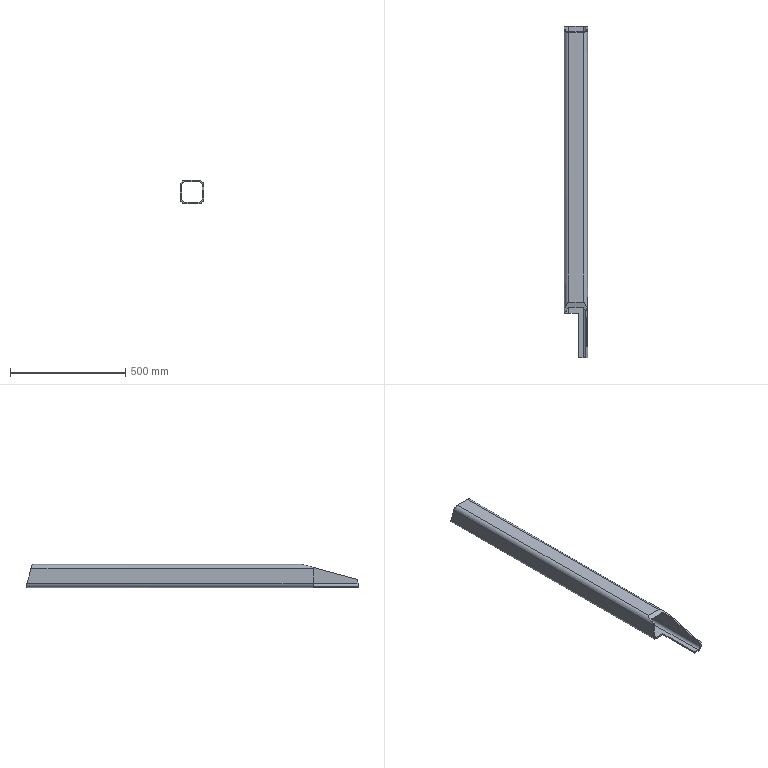Part | SolidWorks | features MirrorStock 1 | 1 solid | 21 faces | box 100 x 1442 x 100 mm | volume 2662768 mm3 | plane 13 | cylinder 8 | commonest cylinder face diameters 26.12 x4 38.12 x4
STEP:
#1=CARTESIAN_POINT('',(-50.,1420.107,30.94));
#2=VERTEX_POINT('',#1);
#3=CARTESIAN_POINT('',(-69.06,1415.,50.));
#4=VERTEX_POINT('',#3);
#5=CARTESIAN_POINT('',(-50.,1420.107,30.94));
#6=CARTESIAN_POINT('',(-50.,1417.115,42.105));
#7=CARTESIAN_POINT('',(-57.895,1415.,50.));
#8=CARTESIAN_POINT('',(-69.06,1415.,50.));
#9=(BOUNDED_CURVE()B_SPLINE_CURVE(3,(#5,#6,#7,#8),.UNSPECIFIED.,.F.,.T.)B_SPLINE_CURVE_WITH_KNOTS((4,4),(4.712,6.283),.UNSPECIFIED.)CURVE()GEOMETRIC_REPRESENTATION_ITEM()RATIONAL_B_SPLINE_CURVE((1.,0.8047,0.8047,1.))REPRESENTATION_ITEM(''));
#10=EDGE_CURVE('',#2,#4,#9,.T.);
#11=ORIENTED_EDGE('',*,*,#10,.T.);
#12=CARTESIAN_POINT('',(-69.06,242.583,50.));
#13=VERTEX_POINT('',#12);
#14=CARTESIAN_POINT('',(-69.06,1500.,50.));
#15=DIRECTION('',(0.,-1.,0.));
#16=VECTOR('',#15,1000.);
#17=LINE('',#14,#16);
#18=EDGE_CURVE('',#4,#13,#17,.T.);
#19=ORIENTED_EDGE('',*,*,#18,.T.);
#20=CARTESIAN_POINT('',(-50.,171.45,30.94));
#21=VERTEX_POINT('',#20);
#22=CARTESIAN_POINT('',(-50.,171.45,30.94));
#23=CARTESIAN_POINT('',(-50.,213.119,42.105));
#24=CARTESIAN_POINT('',(-57.895,242.583,50.));
#25=CARTESIAN_POINT('',(-69.06,242.583,50.));
#26=(BOUNDED_CURVE()B_SPLINE_CURVE(3,(#22,#23,#24,#25),.UNSPECIFIED.,.F.,.T.)B_SPLINE_CURVE_WITH_KNOTS((4,4),(1.571,3.142),.UNSPECIFIED.)CURVE()GEOMETRIC_REPRESENTATION_ITEM()RATIONAL_B_SPLINE_CURVE((1.,0.8047,0.8047,1.))REPRESENTATION_ITEM(''));
#27=EDGE_CURVE('',#21,#13,#26,.T.);
#28=ORIENTED_EDGE('',*,*,#27,.F.);
#29=CARTESIAN_POINT('',(-50.,1500.,30.94));
#30=DIRECTION('',(0.,-1.,0.));
#31=VECTOR('',#30,1000.);
#32=LINE('',#29,#31);
#33=EDGE_CURVE('',#2,#21,#32,.T.);
#34=ORIENTED_EDGE('',*,*,#33,.F.);
#35=EDGE_LOOP('',(#11,#19,#28,#34));
#36=FACE_OUTER_BOUND('',#35,.T.);
#37=CARTESIAN_POINT('',(-69.06,1500.,30.94));
#38=DIRECTION('',(0.,-1.,0.));
#39=DIRECTION('',(0.,0.,-1.));
#40=AXIS2_PLACEMENT_3D('',#37,#38,#39);
#41=CYLINDRICAL_SURFACE('',#40,19.06);
#42=ADVANCED_FACE('',(#36),#41,.T.);
#43=CARTESIAN_POINT('',(-130.94,1415.,50.));
#44=VERTEX_POINT('',#43);
#45=CARTESIAN_POINT('',(-251.,1415.,50.));
#46=DIRECTION('',(1.,0.,0.));
#47=VECTOR('',#46,1000.);
#48=LINE('',#45,#47);
#49=EDGE_CURVE('',#44,#4,#48,.T.);
#50=ORIENTED_EDGE('',*,*,#49,.F.);
#51=CARTESIAN_POINT('',(-130.94,242.583,50.));
#52=VERTEX_POINT('',#51);
#53=CARTESIAN_POINT('',(-130.94,1500.,50.));
#54=DIRECTION('',(0.,-1.,0.));
#55=VECTOR('',#54,1000.);
#56=LINE('',#53,#55);
#57=EDGE_CURVE('',#44,#52,#56,.T.);
#58=ORIENTED_EDGE('',*,*,#57,.T.);
#59=CARTESIAN_POINT('',(37.,242.583,50.));
#60=DIRECTION('',(-1.,0.,0.));
#61=VECTOR('',#60,1000.);
#62=LINE('',#59,#61);
#63=EDGE_CURVE('',#13,#52,#62,.T.);
#64=ORIENTED_EDGE('',*,*,#63,.F.);
#65=ORIENTED_EDGE('',*,*,#18,.F.);
#66=EDGE_LOOP('',(#50,#58,#64,#65));
#67=FACE_OUTER_BOUND('',#66,.T.);
#68=CARTESIAN_POINT('',(-69.06,1500.,50.));
#69=DIRECTION('',(0.,0.,-1.));
#70=DIRECTION('',(1.,0.,0.));
#71=AXIS2_PLACEMENT_3D('',#68,#69,#70);
#72=PLANE('',#71);
#73=ADVANCED_FACE('',(#67),#72,.F.);
#74=CARTESIAN_POINT('',(-150.,1420.107,30.94));
#75=VERTEX_POINT('',#74);
#76=CARTESIAN_POINT('',(-130.94,1415.,50.));
#77=CARTESIAN_POINT('',(-142.105,1415.,50.));
#78=CARTESIAN_POINT('',(-150.,1417.115,42.105));
#79=CARTESIAN_POINT('',(-150.,1420.107,30.94));
#80=(BOUNDED_CURVE()B_SPLINE_CURVE(3,(#76,#77,#78,#79),.UNSPECIFIED.,.F.,.F.)B_SPLINE_CURVE_WITH_KNOTS((4,4),(0.,1.571),.UNSPECIFIED.)CURVE()GEOMETRIC_REPRESENTATION_ITEM()RATIONAL_B_SPLINE_CURVE((1.,0.8047,0.8047,1.))REPRESENTATION_ITEM(''));
#81=EDGE_CURVE('',#44,#75,#80,.T.);
#82=ORIENTED_EDGE('',*,*,#81,.T.);
#83=CARTESIAN_POINT('',(-150.,195.,30.94));
#84=VERTEX_POINT('',#83);
#85=CARTESIAN_POINT('',(-150.,1500.,30.94));
#86=DIRECTION('',(0.,-1.,0.));
#87=VECTOR('',#86,1000.);
#88=LINE('',#85,#87);
#89=EDGE_CURVE('',#75,#84,#88,.T.);
#90=ORIENTED_EDGE('',*,*,#89,.T.);
#91=CARTESIAN_POINT('',(-148.925,195.,37.25));
#92=VERTEX_POINT('',#91);
#93=CARTESIAN_POINT('',(-130.94,195.,30.94));
#94=DIRECTION('',(0.,-1.,0.));
#95=DIRECTION('',(0.,0.,1.));
#96=AXIS2_PLACEMENT_3D('',#93,#94,#95);
#97=CIRCLE('',#96,19.06);
#98=EDGE_CURVE('',#92,#84,#97,.T.);
#99=ORIENTED_EDGE('',*,*,#98,.F.);
#100=CARTESIAN_POINT('',(-130.94,242.583,50.));
#101=CARTESIAN_POINT('',(-139.317,242.583,50.));
#102=CARTESIAN_POINT('',(-146.152,224.502,45.155));
#103=CARTESIAN_POINT('',(-148.925,195.,37.25));
#104=(BOUNDED_CURVE()B_SPLINE_CURVE(3,(#100,#101,#102,#103),.UNSPECIFIED.,.F.,.T.)B_SPLINE_CURVE_WITH_KNOTS((4,4),(3.142,4.375),.UNSPECIFIED.)CURVE()GEOMETRIC_REPRESENTATION_ITEM()RATIONAL_B_SPLINE_CURVE((1.,0.8772,0.8772,1.))REPRESENTATION_ITEM(''));
#105=EDGE_CURVE('',#52,#92,#104,.T.);
#106=ORIENTED_EDGE('',*,*,#105,.F.);
#107=ORIENTED_EDGE('',*,*,#57,.F.);
#108=EDGE_LOOP('',(#82,#90,#99,#106,#107));
#109=FACE_OUTER_BOUND('',#108,.T.);
#110=CARTESIAN_POINT('',(-130.94,1500.,30.94));
#111=DIRECTION('',(0.,-1.,0.));
#112=DIRECTION('',(0.,0.,-1.));
#113=AXIS2_PLACEMENT_3D('',#110,#111,#112);
#114=CYLINDRICAL_SURFACE('',#113,19.06);
#115=ADVANCED_FACE('',(#109),#114,.T.);
#116=CARTESIAN_POINT('',(-150.,1436.688,-30.94));
#117=VERTEX_POINT('',#116);
#118=CARTESIAN_POINT('',(-150.,1440.929,-46.768));
#119=DIRECTION('',(0.,0.2588,-0.9659));
#120=VECTOR('',#119,1000.);
#121=LINE('',#118,#120);
#122=EDGE_CURVE('',#75,#117,#121,.T.);
#123=ORIENTED_EDGE('',*,*,#122,.T.);
#124=CARTESIAN_POINT('',(-150.,195.,-30.94));
#125=VERTEX_POINT('',#124);
#126=CARTESIAN_POINT('',(-150.,1500.,-30.94));
#127=DIRECTION('',(0.,-1.,0.));
#128=VECTOR('',#127,1000.);
#129=LINE('',#126,#128);
#130=EDGE_CURVE('',#117,#125,#129,.T.);
#131=ORIENTED_EDGE('',*,*,#130,.T.);
#132=CARTESIAN_POINT('',(-150.,195.,-30.94));
#133=DIRECTION('',(0.,0.,-1.));
#134=VECTOR('',#133,1000.);
#135=LINE('',#132,#134);
#136=EDGE_CURVE('',#84,#125,#135,.T.);
#137=ORIENTED_EDGE('',*,*,#136,.F.);
#138=ORIENTED_EDGE('',*,*,#89,.F.);
#139=EDGE_LOOP('',(#123,#131,#137,#138));
#140=FACE_OUTER_BOUND('',#139,.T.);
#141=CARTESIAN_POINT('',(-150.,1500.,-30.94));
#142=DIRECTION('',(1.,0.,0.));
#143=DIRECTION('',(0.,0.,1.));
#144=AXIS2_PLACEMENT_3D('',#141,#142,#143);
#145=PLANE('',#144);
#146=ADVANCED_FACE('',(#140),#145,.F.);
#147=CARTESIAN_POINT('',(-130.94,1441.795,-50.));
#148=VERTEX_POINT('',#147);
#149=CARTESIAN_POINT('',(-150.,1436.688,-30.94));
#150=CARTESIAN_POINT('',(-150.,1439.679,-42.105));
#151=CARTESIAN_POINT('',(-142.105,1441.795,-50.));
#152=CARTESIAN_POINT('',(-130.94,1441.795,-50.));
#153=(BOUNDED_CURVE()B_SPLINE_CURVE(3,(#149,#150,#151,#152),.UNSPECIFIED.,.F.,.T.)B_SPLINE_CURVE_WITH_KNOTS((4,4),(1.571,3.142),.UNSPECIFIED.)CURVE()GEOMETRIC_REPRESENTATION_ITEM()RATIONAL_B_SPLINE_CURVE((1.,0.8047,0.8047,1.))REPRESENTATION_ITEM(''));
#154=EDGE_CURVE('',#117,#148,#153,.T.);
#155=ORIENTED_EDGE('',*,*,#154,.T.);
#156=CARTESIAN_POINT('',(-130.94,195.,-50.));
#157=VERTEX_POINT('',#156);
#158=CARTESIAN_POINT('',(-130.94,1500.,-50.));
#159=DIRECTION('',(0.,-1.,0.));
#160=VECTOR('',#159,1000.);
#161=LINE('',#158,#160);
#162=EDGE_CURVE('',#148,#157,#161,.T.);
#163=ORIENTED_EDGE('',*,*,#162,.T.);
#164=CARTESIAN_POINT('',(-130.94,195.,-30.94));
#165=DIRECTION('',(0.,-1.,0.));
#166=DIRECTION('',(0.,0.,1.));
#167=AXIS2_PLACEMENT_3D('',#164,#165,#166);
#168=CIRCLE('',#167,19.06);
#169=EDGE_CURVE('',#125,#157,#168,.T.);
#170=ORIENTED_EDGE('',*,*,#169,.F.);
#171=ORIENTED_EDGE('',*,*,#130,.F.);
#172=EDGE_LOOP('',(#155,#163,#170,#171));
#173=FACE_OUTER_BOUND('',#172,.T.);
#174=CARTESIAN_POINT('',(-130.94,1500.,-30.94));
#175=DIRECTION('',(0.,-1.,0.));
#176=DIRECTION('',(0.,0.,-1.));
#177=AXIS2_PLACEMENT_3D('',#174,#175,#176);
#178=CYLINDRICAL_SURFACE('',#177,19.06);
#179=ADVANCED_FACE('',(#173),#178,.T.);
#180=CARTESIAN_POINT('',(-69.06,1441.795,-50.));
#181=VERTEX_POINT('',#180);
#182=CARTESIAN_POINT('',(-251.,1441.795,-50.));
#183=DIRECTION('',(1.,0.,0.));
#184=VECTOR('',#183,1000.);
#185=LINE('',#182,#184);
#186=EDGE_CURVE('',#148,#181,#185,.T.);
#187=ORIENTED_EDGE('',*,*,#186,.T.);
#188=CARTESIAN_POINT('',(-69.06,0.,-50.));
#189=VERTEX_POINT('',#188);
#190=CARTESIAN_POINT('',(-69.06,1500.,-50.));
#191=DIRECTION('',(0.,-1.,0.));
#192=VECTOR('',#191,1000.);
#193=LINE('',#190,#192);
#194=EDGE_CURVE('',#181,#189,#193,.T.);
#195=ORIENTED_EDGE('',*,*,#194,.T.);
#196=CARTESIAN_POINT('',(-90.,0.,-50.));
#197=VERTEX_POINT('',#196);
#198=CARTESIAN_POINT('',(-130.94,0.,-50.));
#199=DIRECTION('',(1.,0.,0.));
#200=VECTOR('',#199,1000.);
#201=LINE('',#198,#200);
#202=EDGE_CURVE('',#197,#189,#201,.T.);
#203=ORIENTED_EDGE('',*,*,#202,.F.);
#204=CARTESIAN_POINT('',(-90.,195.,-50.));
#205=VERTEX_POINT('',#204);
#206=CARTESIAN_POINT('',(-90.,1500.,-50.));
#207=DIRECTION('',(0.,-1.,0.));
#208=VECTOR('',#207,1000.);
#209=LINE('',#206,#208);
#210=EDGE_CURVE('',#205,#197,#209,.T.);
#211=ORIENTED_EDGE('',*,*,#210,.F.);
#212=CARTESIAN_POINT('',(-130.94,195.,-50.));
#213=DIRECTION('',(1.,0.,0.));
#214=VECTOR('',#213,1000.);
#215=LINE('',#212,#214);
#216=EDGE_CURVE('',#157,#205,#215,.T.);
#217=ORIENTED_EDGE('',*,*,#216,.F.);
#218=ORIENTED_EDGE('',*,*,#162,.F.);
#219=EDGE_LOOP('',(#187,#195,#203,#211,#217,#218));
#220=FACE_OUTER_BOUND('',#219,.T.);
#221=CARTESIAN_POINT('',(-130.94,1500.,-50.));
#222=DIRECTION('',(0.,0.,1.));
#223=DIRECTION('',(-1.,0.,0.));
#224=AXIS2_PLACEMENT_3D('',#221,#222,#223);
#225=PLANE('',#224);
#226=ADVANCED_FACE('',(#220),#225,.F.);
#227=CARTESIAN_POINT('',(-50.,1436.688,-30.94));
#228=VERTEX_POINT('',#227);
#229=CARTESIAN_POINT('',(-69.06,1441.795,-50.));
#230=CARTESIAN_POINT('',(-57.895,1441.795,-50.));
#231=CARTESIAN_POINT('',(-50.,1439.679,-42.105));
#232=CARTESIAN_POINT('',(-50.,1436.688,-30.94));
#233=(BOUNDED_CURVE()B_SPLINE_CURVE(3,(#229,#230,#231,#232),.UNSPECIFIED.,.F.,.T.)B_SPLINE_CURVE_WITH_KNOTS((4,4),(3.142,4.712),.UNSPECIFIED.)CURVE()GEOMETRIC_REPRESENTATION_ITEM()RATIONAL_B_SPLINE_CURVE((1.,0.8047,0.8047,1.))REPRESENTATION_ITEM(''));
#234=EDGE_CURVE('',#181,#228,#233,.T.);
#235=ORIENTED_EDGE('',*,*,#234,.T.);
#236=CARTESIAN_POINT('',(-50.,0.,-30.94));
#237=VERTEX_POINT('',#236);
#238=CARTESIAN_POINT('',(-50.,1500.,-30.94));
#239=DIRECTION('',(0.,-1.,0.));
#240=VECTOR('',#239,1000.);
#241=LINE('',#238,#240);
#242=EDGE_CURVE('',#228,#237,#241,.T.);
#243=ORIENTED_EDGE('',*,*,#242,.T.);
#244=CARTESIAN_POINT('',(-69.06,0.,-30.94));
#245=DIRECTION('',(0.,-1.,0.));
#246=DIRECTION('',(0.,0.,1.));
#247=AXIS2_PLACEMENT_3D('',#244,#245,#246);
#248=CIRCLE('',#247,19.06);
#249=EDGE_CURVE('',#189,#237,#248,.T.);
#250=ORIENTED_EDGE('',*,*,#249,.F.);
#251=ORIENTED_EDGE('',*,*,#194,.F.);
#252=EDGE_LOOP('',(#235,#243,#250,#251));
#253=FACE_OUTER_BOUND('',#252,.T.);
#254=CARTESIAN_POINT('',(-69.06,1500.,-30.94));
#255=DIRECTION('',(0.,-1.,0.));
#256=DIRECTION('',(0.,0.,-1.));
#257=AXIS2_PLACEMENT_3D('',#254,#255,#256);
#258=CYLINDRICAL_SURFACE('',#257,19.06);
#259=ADVANCED_FACE('',(#253),#258,.T.);
#260=CARTESIAN_POINT('',(-130.94,1416.608,44.));
#261=VERTEX_POINT('',#260);
#262=CARTESIAN_POINT('',(-130.94,220.191,44.));
#263=VERTEX_POINT('',#262);
#264=CARTESIAN_POINT('',(-130.94,1500.,44.));
#265=DIRECTION('',(0.,-1.,0.));
#266=VECTOR('',#265,1000.);
#267=LINE('',#264,#266);
#268=EDGE_CURVE('',#261,#263,#267,.T.);
#269=ORIENTED_EDGE('',*,*,#268,.T.);
#270=CARTESIAN_POINT('',(-142.374,195.,37.25));
#271=VERTEX_POINT('',#270);
#272=CARTESIAN_POINT('',(-130.94,220.191,44.));
#273=CARTESIAN_POINT('',(-135.818,220.191,44.));
#274=CARTESIAN_POINT('',(-140.018,210.937,41.521));
#275=CARTESIAN_POINT('',(-142.374,195.,37.25));
#276=(BOUNDED_CURVE()B_SPLINE_CURVE(3,(#272,#273,#274,#275),.UNSPECIFIED.,.F.,.T.)B_SPLINE_CURVE_WITH_KNOTS((4,4),(3.142,4.208),.UNSPECIFIED.)CURVE()GEOMETRIC_REPRESENTATION_ITEM()RATIONAL_B_SPLINE_CURVE((1.,0.9074,0.9074,1.))REPRESENTATION_ITEM(''));
#277=EDGE_CURVE('',#263,#271,#276,.T.);
#278=ORIENTED_EDGE('',*,*,#277,.T.);
#279=CARTESIAN_POINT('',(-144.,195.,30.94));
#280=VERTEX_POINT('',#279);
#281=CARTESIAN_POINT('',(-130.94,195.,30.94));
#282=DIRECTION('',(0.,-1.,0.));
#283=DIRECTION('',(0.,0.,1.));
#284=AXIS2_PLACEMENT_3D('',#281,#282,#283);
#285=CIRCLE('',#284,13.06);
#286=EDGE_CURVE('',#271,#280,#285,.T.);
#287=ORIENTED_EDGE('',*,*,#286,.T.);
#288=CARTESIAN_POINT('',(-144.,1420.107,30.94));
#289=VERTEX_POINT('',#288);
#290=CARTESIAN_POINT('',(-144.,1500.,30.94));
#291=DIRECTION('',(0.,-1.,0.));
#292=VECTOR('',#291,1000.);
#293=LINE('',#290,#292);
#294=EDGE_CURVE('',#289,#280,#293,.T.);
#295=ORIENTED_EDGE('',*,*,#294,.F.);
#296=CARTESIAN_POINT('',(-130.94,1416.608,44.));
#297=CARTESIAN_POINT('',(-138.59,1416.608,44.));
#298=CARTESIAN_POINT('',(-144.,1418.057,38.59));
#299=CARTESIAN_POINT('',(-144.,1420.107,30.94));
#300=(BOUNDED_CURVE()B_SPLINE_CURVE(3,(#296,#297,#298,#299),.UNSPECIFIED.,.F.,.T.)B_SPLINE_CURVE_WITH_KNOTS((4,4),(0.,1.571),.UNSPECIFIED.)CURVE()GEOMETRIC_REPRESENTATION_ITEM()RATIONAL_B_SPLINE_CURVE((1.,0.8047,0.8047,1.))REPRESENTATION_ITEM(''));
#301=EDGE_CURVE('',#261,#289,#300,.T.);
#302=ORIENTED_EDGE('',*,*,#301,.F.);
#303=EDGE_LOOP('',(#269,#278,#287,#295,#302));
#304=FACE_OUTER_BOUND('',#303,.T.);
#305=CARTESIAN_POINT('',(-130.94,1500.,30.94));
#306=DIRECTION('',(0.,-1.,0.));
#307=DIRECTION('',(0.,0.,-1.));
#308=AXIS2_PLACEMENT_3D('',#305,#306,#307);
#309=CYLINDRICAL_SURFACE('',#308,13.06);
#310=ADVANCED_FACE('',(#304),#309,.F.);
#311=CARTESIAN_POINT('',(-69.06,1416.608,44.));
#312=VERTEX_POINT('',#311);
#313=CARTESIAN_POINT('',(-69.06,220.191,44.));
#314=VERTEX_POINT('',#313);
#315=CARTESIAN_POINT('',(-69.06,1500.,44.));
#316=DIRECTION('',(0.,-1.,0.));
#317=VECTOR('',#316,1000.);
#318=LINE('',#315,#317);
#319=EDGE_CURVE('',#312,#314,#318,.T.);
#320=ORIENTED_EDGE('',*,*,#319,.T.);
#321=CARTESIAN_POINT('',(-69.06,220.191,44.));
#322=DIRECTION('',(-1.,0.,0.));
#323=VECTOR('',#322,1000.);
#324=LINE('',#321,#323);
#325=EDGE_CURVE('',#314,#263,#324,.T.);
#326=ORIENTED_EDGE('',*,*,#325,.T.);
#327=ORIENTED_EDGE('',*,*,#268,.F.);
#328=CARTESIAN_POINT('',(-69.06,1416.608,44.));
#329=DIRECTION('',(-1.,0.,0.));
#330=VECTOR('',#329,1000.);
#331=LINE('',#328,#330);
#332=EDGE_CURVE('',#312,#261,#331,.T.);
#333=ORIENTED_EDGE('',*,*,#332,.F.);
#334=EDGE_LOOP('',(#320,#326,#327,#333));
#335=FACE_OUTER_BOUND('',#334,.T.);
#336=CARTESIAN_POINT('',(-69.06,1500.,44.));
#337=DIRECTION('',(0.,0.,-1.));
#338=DIRECTION('',(1.,0.,0.));
#339=AXIS2_PLACEMENT_3D('',#336,#337,#338);
#340=PLANE('',#339);
#341=ADVANCED_FACE('',(#335),#340,.T.);
#342=CARTESIAN_POINT('',(-56.,1420.107,30.94));
#343=VERTEX_POINT('',#342);
#344=CARTESIAN_POINT('',(-56.,171.45,30.94));
#345=VERTEX_POINT('',#344);
#346=CARTESIAN_POINT('',(-56.,1500.,30.94));
#347=DIRECTION('',(0.,-1.,0.));
#348=VECTOR('',#347,1000.);
#349=LINE('',#346,#348);
#350=EDGE_CURVE('',#343,#345,#349,.T.);
#351=ORIENTED_EDGE('',*,*,#350,.T.);
#352=CARTESIAN_POINT('',(-56.,171.45,30.94));
#353=CARTESIAN_POINT('',(-56.,200.002,38.59));
#354=CARTESIAN_POINT('',(-61.41,220.191,44.));
#355=CARTESIAN_POINT('',(-69.06,220.191,44.));
#356=(BOUNDED_CURVE()B_SPLINE_CURVE(3,(#352,#353,#354,#355),.UNSPECIFIED.,.F.,.F.)B_SPLINE_CURVE_WITH_KNOTS((4,4),(1.571,3.142),.UNSPECIFIED.)CURVE()GEOMETRIC_REPRESENTATION_ITEM()RATIONAL_B_SPLINE_CURVE((1.,0.8047,0.8047,1.))REPRESENTATION_ITEM(''));
#357=EDGE_CURVE('',#345,#314,#356,.T.);
#358=ORIENTED_EDGE('',*,*,#357,.T.);
#359=ORIENTED_EDGE('',*,*,#319,.F.);
#360=CARTESIAN_POINT('',(-56.,1420.107,30.94));
#361=CARTESIAN_POINT('',(-56.,1418.057,38.59));
#362=CARTESIAN_POINT('',(-61.41,1416.608,44.));
#363=CARTESIAN_POINT('',(-69.06,1416.608,44.));
#364=(BOUNDED_CURVE()B_SPLINE_CURVE(3,(#360,#361,#362,#363),.UNSPECIFIED.,.F.,.F.)B_SPLINE_CURVE_WITH_KNOTS((4,4),(4.712,6.283),.UNSPECIFIED.)CURVE()GEOMETRIC_REPRESENTATION_ITEM()RATIONAL_B_SPLINE_CURVE((1.,0.8047,0.8047,1.))REPRESENTATION_ITEM(''));
#365=EDGE_CURVE('',#343,#312,#364,.T.);
#366=ORIENTED_EDGE('',*,*,#365,.F.);
#367=EDGE_LOOP('',(#351,#358,#359,#366));
#368=FACE_OUTER_BOUND('',#367,.T.);
#369=CARTESIAN_POINT('',(-69.06,1500.,30.94));
#370=DIRECTION('',(0.,-1.,0.));
#371=DIRECTION('',(0.,0.,-1.));
#372=AXIS2_PLACEMENT_3D('',#369,#370,#371);
#373=CYLINDRICAL_SURFACE('',#372,13.06);
#374=ADVANCED_FACE('',(#368),#373,.F.);
#375=CARTESIAN_POINT('',(-56.,1436.688,-30.94));
#376=VERTEX_POINT('',#375);
#377=CARTESIAN_POINT('',(-56.,0.,-30.94));
#378=VERTEX_POINT('',#377);
#379=CARTESIAN_POINT('',(-56.,1500.,-30.94));
#380=DIRECTION('',(0.,-1.,0.));
#381=VECTOR('',#380,1000.);
#382=LINE('',#379,#381);
#383=EDGE_CURVE('',#376,#378,#382,.T.);
#384=ORIENTED_EDGE('',*,*,#383,.T.);
#385=CARTESIAN_POINT('',(-56.,0.,-15.));
#386=VERTEX_POINT('',#385);
#387=CARTESIAN_POINT('',(-56.,0.,30.94));
#388=DIRECTION('',(0.,0.,1.));
#389=VECTOR('',#388,1000.);
#390=LINE('',#387,#389);
#391=EDGE_CURVE('',#378,#386,#390,.T.);
#392=ORIENTED_EDGE('',*,*,#391,.T.);
#393=CARTESIAN_POINT('',(-56.,1411.004,363.077));
#394=DIRECTION('',(0.,0.9659,0.2588));
#395=VECTOR('',#394,1000.);
#396=LINE('',#393,#395);
#397=EDGE_CURVE('',#386,#345,#396,.T.);
#398=ORIENTED_EDGE('',*,*,#397,.T.);
#399=ORIENTED_EDGE('',*,*,#350,.F.);
#400=CARTESIAN_POINT('',(-56.,1425.459,10.967));
#401=DIRECTION('',(0.,-0.2588,0.9659));
#402=VECTOR('',#401,1000.);
#403=LINE('',#400,#402);
#404=EDGE_CURVE('',#376,#343,#403,.T.);
#405=ORIENTED_EDGE('',*,*,#404,.F.);
#406=EDGE_LOOP('',(#384,#392,#398,#399,#405));
#407=FACE_OUTER_BOUND('',#406,.T.);
#408=CARTESIAN_POINT('',(-56.,1500.,30.94));
#409=DIRECTION('',(-1.,0.,0.));
#410=DIRECTION('',(0.,0.,-1.));
#411=AXIS2_PLACEMENT_3D('',#408,#409,#410);
#412=PLANE('',#411);
#413=ADVANCED_FACE('',(#407),#412,.T.);
#414=CARTESIAN_POINT('',(-69.06,1440.187,-44.));
#415=VERTEX_POINT('',#414);
#416=CARTESIAN_POINT('',(-69.06,0.,-44.));
#417=VERTEX_POINT('',#416);
#418=CARTESIAN_POINT('',(-69.06,1500.,-44.));
#419=DIRECTION('',(0.,-1.,0.));
#420=VECTOR('',#419,1000.);
#421=LINE('',#418,#420);
#422=EDGE_CURVE('',#415,#417,#421,.T.);
#423=ORIENTED_EDGE('',*,*,#422,.T.);
#424=CARTESIAN_POINT('',(-69.06,0.,-30.94));
#425=DIRECTION('',(0.,-1.,0.));
#426=DIRECTION('',(0.,0.,1.));
#427=AXIS2_PLACEMENT_3D('',#424,#425,#426);
#428=CIRCLE('',#427,13.06);
#429=EDGE_CURVE('',#417,#378,#428,.T.);
#430=ORIENTED_EDGE('',*,*,#429,.T.);
#431=ORIENTED_EDGE('',*,*,#383,.F.);
#432=CARTESIAN_POINT('',(-69.06,1440.187,-44.));
#433=CARTESIAN_POINT('',(-61.41,1440.187,-44.));
#434=CARTESIAN_POINT('',(-56.,1438.738,-38.59));
#435=CARTESIAN_POINT('',(-56.,1436.688,-30.94));
#436=(BOUNDED_CURVE()B_SPLINE_CURVE(3,(#432,#433,#434,#435),.UNSPECIFIED.,.F.,.T.)B_SPLINE_CURVE_WITH_KNOTS((4,4),(3.142,4.712),.UNSPECIFIED.)CURVE()GEOMETRIC_REPRESENTATION_ITEM()RATIONAL_B_SPLINE_CURVE((1.,0.8047,0.8047,1.))REPRESENTATION_ITEM(''));
#437=EDGE_CURVE('',#415,#376,#436,.T.);
#438=ORIENTED_EDGE('',*,*,#437,.F.);
#439=EDGE_LOOP('',(#423,#430,#431,#438));
#440=FACE_OUTER_BOUND('',#439,.T.);
#441=CARTESIAN_POINT('',(-69.06,1500.,-30.94));
#442=DIRECTION('',(0.,-1.,0.));
#443=DIRECTION('',(0.,0.,-1.));
#444=AXIS2_PLACEMENT_3D('',#441,#442,#443);
#445=CYLINDRICAL_SURFACE('',#444,13.06);
#446=ADVANCED_FACE('',(#440),#445,.F.);
#447=CARTESIAN_POINT('',(-130.94,1440.187,-44.));
#448=VERTEX_POINT('',#447);
#449=CARTESIAN_POINT('',(-130.94,195.,-44.));
#450=VERTEX_POINT('',#449);
#451=CARTESIAN_POINT('',(-130.94,1500.,-44.));
#452=DIRECTION('',(0.,-1.,0.));
#453=VECTOR('',#452,1000.);
#454=LINE('',#451,#453);
#455=EDGE_CURVE('',#448,#450,#454,.T.);
#456=ORIENTED_EDGE('',*,*,#455,.T.);
#457=CARTESIAN_POINT('',(-90.,195.,-44.));
#458=VERTEX_POINT('',#457);
#459=CARTESIAN_POINT('',(-130.94,195.,-44.));
#460=DIRECTION('',(1.,0.,0.));
#461=VECTOR('',#460,1000.);
#462=LINE('',#459,#461);
#463=EDGE_CURVE('',#450,#458,#462,.T.);
#464=ORIENTED_EDGE('',*,*,#463,.T.);
#465=CARTESIAN_POINT('',(-90.,0.,-44.));
#466=VERTEX_POINT('',#465);
#467=CARTESIAN_POINT('',(-90.,1500.,-44.));
#468=DIRECTION('',(0.,-1.,0.));
#469=VECTOR('',#468,1000.);
#470=LINE('',#467,#469);
#471=EDGE_CURVE('',#458,#466,#470,.T.);
#472=ORIENTED_EDGE('',*,*,#471,.T.);
#473=CARTESIAN_POINT('',(-130.94,0.,-44.));
#474=DIRECTION('',(1.,0.,0.));
#475=VECTOR('',#474,1000.);
#476=LINE('',#473,#475);
#477=EDGE_CURVE('',#466,#417,#476,.T.);
#478=ORIENTED_EDGE('',*,*,#477,.T.);
#479=ORIENTED_EDGE('',*,*,#422,.F.);
#480=CARTESIAN_POINT('',(-130.94,1440.187,-44.));
#481=DIRECTION('',(1.,0.,0.));
#482=VECTOR('',#481,1000.);
#483=LINE('',#480,#482);
#484=EDGE_CURVE('',#448,#415,#483,.T.);
#485=ORIENTED_EDGE('',*,*,#484,.F.);
#486=EDGE_LOOP('',(#456,#464,#472,#478,#479,#485));
#487=FACE_OUTER_BOUND('',#486,.T.);
#488=CARTESIAN_POINT('',(-130.94,1500.,-44.));
#489=DIRECTION('',(0.,0.,1.));
#490=DIRECTION('',(-1.,0.,0.));
#491=AXIS2_PLACEMENT_3D('',#488,#489,#490);
#492=PLANE('',#491);
#493=ADVANCED_FACE('',(#487),#492,.T.);
#494=CARTESIAN_POINT('',(-144.,1436.688,-30.94));
#495=VERTEX_POINT('',#494);
#496=CARTESIAN_POINT('',(-144.,195.,-30.94));
#497=VERTEX_POINT('',#496);
#498=CARTESIAN_POINT('',(-144.,1500.,-30.94));
#499=DIRECTION('',(0.,-1.,0.));
#500=VECTOR('',#499,1000.);
#501=LINE('',#498,#500);
#502=EDGE_CURVE('',#495,#497,#501,.T.);
#503=ORIENTED_EDGE('',*,*,#502,.T.);
#504=CARTESIAN_POINT('',(-130.94,195.,-30.94));
#505=DIRECTION('',(0.,-1.,0.));
#506=DIRECTION('',(0.,0.,1.));
#507=AXIS2_PLACEMENT_3D('',#504,#505,#506);
#508=CIRCLE('',#507,13.06);
#509=EDGE_CURVE('',#497,#450,#508,.T.);
#510=ORIENTED_EDGE('',*,*,#509,.T.);
#511=ORIENTED_EDGE('',*,*,#455,.F.);
#512=CARTESIAN_POINT('',(-144.,1436.688,-30.94));
#513=CARTESIAN_POINT('',(-144.,1438.738,-38.59));
#514=CARTESIAN_POINT('',(-138.59,1440.187,-44.));
#515=CARTESIAN_POINT('',(-130.94,1440.187,-44.));
#516=(BOUNDED_CURVE()B_SPLINE_CURVE(3,(#512,#513,#514,#515),.UNSPECIFIED.,.F.,.T.)B_SPLINE_CURVE_WITH_KNOTS((4,4),(1.571,3.142),.UNSPECIFIED.)CURVE()GEOMETRIC_REPRESENTATION_ITEM()RATIONAL_B_SPLINE_CURVE((1.,0.8047,0.8047,1.))REPRESENTATION_ITEM(''));
#517=EDGE_CURVE('',#495,#448,#516,.T.);
#518=ORIENTED_EDGE('',*,*,#517,.F.);
#519=EDGE_LOOP('',(#503,#510,#511,#518));
#520=FACE_OUTER_BOUND('',#519,.T.);
#521=CARTESIAN_POINT('',(-130.94,1500.,-30.94));
#522=DIRECTION('',(0.,-1.,0.));
#523=DIRECTION('',(0.,0.,-1.));
#524=AXIS2_PLACEMENT_3D('',#521,#522,#523);
#525=CYLINDRICAL_SURFACE('',#524,13.06);
#526=ADVANCED_FACE('',(#520),#525,.F.);
#527=ORIENTED_EDGE('',*,*,#294,.T.);
#528=CARTESIAN_POINT('',(-144.,195.,-30.94));
#529=DIRECTION('',(0.,0.,-1.));
#530=VECTOR('',#529,1000.);
#531=LINE('',#528,#530);
#532=EDGE_CURVE('',#280,#497,#531,.T.);
#533=ORIENTED_EDGE('',*,*,#532,.T.);
#534=ORIENTED_EDGE('',*,*,#502,.F.);
#535=CARTESIAN_POINT('',(-144.,1440.929,-46.768));
#536=DIRECTION('',(0.,0.2588,-0.9659));
#537=VECTOR('',#536,1000.);
#538=LINE('',#535,#537);
#539=EDGE_CURVE('',#289,#495,#538,.T.);
#540=ORIENTED_EDGE('',*,*,#539,.F.);
#541=EDGE_LOOP('',(#527,#533,#534,#540));
#542=FACE_OUTER_BOUND('',#541,.T.);
#543=CARTESIAN_POINT('',(-144.,1500.,-30.94));
#544=DIRECTION('',(1.,0.,0.));
#545=DIRECTION('',(0.,0.,1.));
#546=AXIS2_PLACEMENT_3D('',#543,#544,#545);
#547=PLANE('',#546);
#548=ADVANCED_FACE('',(#542),#547,.T.);
#549=CARTESIAN_POINT('',(-50.,1425.459,10.967));
#550=DIRECTION('',(0.,-0.2588,0.9659));
#551=VECTOR('',#550,1000.);
#552=LINE('',#549,#551);
#553=EDGE_CURVE('',#228,#2,#552,.T.);
#554=ORIENTED_EDGE('',*,*,#553,.T.);
#555=ORIENTED_EDGE('',*,*,#33,.T.);
#556=CARTESIAN_POINT('',(-50.,0.,-15.));
#557=VERTEX_POINT('',#556);
#558=CARTESIAN_POINT('',(-50.,1411.004,363.077));
#559=DIRECTION('',(0.,0.9659,0.2588));
#560=VECTOR('',#559,1000.);
#561=LINE('',#558,#560);
#562=EDGE_CURVE('',#557,#21,#561,.T.);
#563=ORIENTED_EDGE('',*,*,#562,.F.);
#564=CARTESIAN_POINT('',(-50.,0.,30.94));
#565=DIRECTION('',(0.,0.,1.));
#566=VECTOR('',#565,1000.);
#567=LINE('',#564,#566);
#568=EDGE_CURVE('',#237,#557,#567,.T.);
#569=ORIENTED_EDGE('',*,*,#568,.F.);
#570=ORIENTED_EDGE('',*,*,#242,.F.);
#571=EDGE_LOOP('',(#554,#555,#563,#569,#570));
#572=FACE_OUTER_BOUND('',#571,.T.);
#573=CARTESIAN_POINT('',(-50.,1500.,30.94));
#574=DIRECTION('',(-1.,0.,0.));
#575=DIRECTION('',(0.,0.,-1.));
#576=AXIS2_PLACEMENT_3D('',#573,#574,#575);
#577=PLANE('',#576);
#578=ADVANCED_FACE('',(#572),#577,.F.);
#579=ORIENTED_EDGE('',*,*,#202,.T.);
#580=ORIENTED_EDGE('',*,*,#249,.T.);
#581=ORIENTED_EDGE('',*,*,#568,.T.);
#582=CARTESIAN_POINT('',(-69.06,0.,-15.));
#583=DIRECTION('',(1.,0.,0.));
#584=VECTOR('',#583,1000.);
#585=LINE('',#582,#584);
#586=EDGE_CURVE('',#386,#557,#585,.T.);
#587=ORIENTED_EDGE('',*,*,#586,.F.);
#588=ORIENTED_EDGE('',*,*,#391,.F.);
#589=ORIENTED_EDGE('',*,*,#429,.F.);
#590=ORIENTED_EDGE('',*,*,#477,.F.);
#591=CARTESIAN_POINT('',(-90.,0.,30.94));
#592=DIRECTION('',(0.,0.,1.));
#593=VECTOR('',#592,1000.);
#594=LINE('',#591,#593);
#595=EDGE_CURVE('',#197,#466,#594,.T.);
#596=ORIENTED_EDGE('',*,*,#595,.F.);
#597=EDGE_LOOP('',(#579,#580,#581,#587,#588,#589,#590,#596));
#598=FACE_OUTER_BOUND('',#597,.T.);
#599=CARTESIAN_POINT('',(-69.06,0.,30.94));
#600=DIRECTION('',(0.,1.,0.));
#601=DIRECTION('',(0.,0.,1.));
#602=AXIS2_PLACEMENT_3D('',#599,#600,#601);
#603=PLANE('',#602);
#604=ADVANCED_FACE('',(#598),#603,.F.);
#605=ORIENTED_EDGE('',*,*,#277,.F.);
#606=ORIENTED_EDGE('',*,*,#325,.F.);
#607=ORIENTED_EDGE('',*,*,#357,.F.);
#608=ORIENTED_EDGE('',*,*,#397,.F.);
#609=ORIENTED_EDGE('',*,*,#586,.T.);
#610=ORIENTED_EDGE('',*,*,#562,.T.);
#611=ORIENTED_EDGE('',*,*,#27,.T.);
#612=ORIENTED_EDGE('',*,*,#63,.T.);
#613=ORIENTED_EDGE('',*,*,#105,.T.);
#614=CARTESIAN_POINT('',(37.,195.,37.25));
#615=DIRECTION('',(-1.,0.,0.));
#616=VECTOR('',#615,1000.);
#617=LINE('',#614,#616);
#618=EDGE_CURVE('',#271,#92,#617,.T.);
#619=ORIENTED_EDGE('',*,*,#618,.F.);
#620=EDGE_LOOP('',(#605,#606,#607,#608,#609,#610,#611,#612,#613,#619));
#621=FACE_OUTER_BOUND('',#620,.T.);
#622=CARTESIAN_POINT('',(37.,0.,-15.));
#623=DIRECTION('',(0.,0.2588,-0.9659));
#624=DIRECTION('',(0.,0.9659,0.2588));
#625=AXIS2_PLACEMENT_3D('',#622,#623,#624);
#626=PLANE('',#625);
#627=ADVANCED_FACE('',(#621),#626,.F.);
#628=CARTESIAN_POINT('',(-90.,195.,-99.));
#629=DIRECTION('',(0.,0.,1.));
#630=VECTOR('',#629,1000.);
#631=LINE('',#628,#630);
#632=EDGE_CURVE('',#205,#458,#631,.T.);
#633=ORIENTED_EDGE('',*,*,#632,.F.);
#634=ORIENTED_EDGE('',*,*,#210,.T.);
#635=ORIENTED_EDGE('',*,*,#595,.T.);
#636=ORIENTED_EDGE('',*,*,#471,.F.);
#637=EDGE_LOOP('',(#633,#634,#635,#636));
#638=FACE_OUTER_BOUND('',#637,.T.);
#639=CARTESIAN_POINT('',(-90.,195.,-99.));
#640=DIRECTION('',(1.,0.,0.));
#641=DIRECTION('',(0.,-1.,0.));
#642=AXIS2_PLACEMENT_3D('',#639,#640,#641);
#643=PLANE('',#642);
#644=ADVANCED_FACE('',(#638),#643,.F.);
#645=ORIENTED_EDGE('',*,*,#169,.T.);
#646=ORIENTED_EDGE('',*,*,#216,.T.);
#647=ORIENTED_EDGE('',*,*,#632,.T.);
#648=ORIENTED_EDGE('',*,*,#463,.F.);
#649=ORIENTED_EDGE('',*,*,#509,.F.);
#650=ORIENTED_EDGE('',*,*,#532,.F.);
#651=ORIENTED_EDGE('',*,*,#286,.F.);
#652=ORIENTED_EDGE('',*,*,#618,.T.);
#653=ORIENTED_EDGE('',*,*,#98,.T.);
#654=ORIENTED_EDGE('',*,*,#136,.T.);
#655=EDGE_LOOP('',(#645,#646,#647,#648,#649,#650,#651,#652,#653,#654));
#656=FACE_OUTER_BOUND('',#655,.T.);
#657=CARTESIAN_POINT('',(-90.,195.,-99.));
#658=DIRECTION('',(0.,1.,0.));
#659=DIRECTION('',(0.,0.,1.));
#660=AXIS2_PLACEMENT_3D('',#657,#658,#659);
#661=PLANE('',#660);
#662=ADVANCED_FACE('',(#656),#661,.F.);
#663=ORIENTED_EDGE('',*,*,#332,.T.);
#664=ORIENTED_EDGE('',*,*,#301,.T.);
#665=ORIENTED_EDGE('',*,*,#539,.T.);
#666=ORIENTED_EDGE('',*,*,#517,.T.);
#667=ORIENTED_EDGE('',*,*,#484,.T.);
#668=ORIENTED_EDGE('',*,*,#437,.T.);
#669=ORIENTED_EDGE('',*,*,#404,.T.);
#670=ORIENTED_EDGE('',*,*,#365,.T.);
#671=EDGE_LOOP('',(#663,#664,#665,#666,#667,#668,#669,#670));
#672=FACE_BOUND('',#671,.T.);
#673=ORIENTED_EDGE('',*,*,#81,.F.);
#674=ORIENTED_EDGE('',*,*,#49,.T.);
#675=ORIENTED_EDGE('',*,*,#10,.F.);
#676=ORIENTED_EDGE('',*,*,#553,.F.);
#677=ORIENTED_EDGE('',*,*,#234,.F.);
#678=ORIENTED_EDGE('',*,*,#186,.F.);
#679=ORIENTED_EDGE('',*,*,#154,.F.);
#680=ORIENTED_EDGE('',*,*,#122,.F.);
#681=EDGE_LOOP('',(#673,#674,#675,#676,#677,#678,#679,#680));
#682=FACE_OUTER_BOUND('',#681,.T.);
#683=CARTESIAN_POINT('',(-251.,1415.,50.));
#684=DIRECTION('',(0.,0.9659,0.2588));
#685=DIRECTION('',(0.,-0.2588,0.9659));
#686=AXIS2_PLACEMENT_3D('',#683,#684,#685);
#687=PLANE('',#686);
#688=ADVANCED_FACE('',(#672,#682),#687,.T.);
#689=CLOSED_SHELL('',(#42,#73,#115,#146,#179,#226,#259,#310,#341,#374,#413,#446,#493,#526,#548,#578,#604,#627,#644,#662,#688));
#690=MANIFOLD_SOLID_BREP('',#689);
#691=CARTESIAN_POINT('',(0.,0.,0.));
#692=DIRECTION('',(0.,0.,1.));
#693=DIRECTION('',(1.,0.,0.));
#694=AXIS2_PLACEMENT_3D('',#691,#692,#693);
#695=(LENGTH_UNIT()NAMED_UNIT(*)SI_UNIT(.MILLI.,.METRE.));
#696=UNCERTAINTY_MEASURE_WITH_UNIT(LENGTH_MEASURE(0.00001),#695,'','');
#697=(NAMED_UNIT(*)PLANE_ANGLE_UNIT()SI_UNIT($,.RADIAN.));
#698=(NAMED_UNIT(*)SI_UNIT($,.STERADIAN.)SOLID_ANGLE_UNIT());
#699=(GEOMETRIC_REPRESENTATION_CONTEXT(3)GLOBAL_UNCERTAINTY_ASSIGNED_CONTEXT((#696))GLOBAL_UNIT_ASSIGNED_CONTEXT((#695,#697,#698))REPRESENTATION_CONTEXT('',''));
#700=ADVANCED_BREP_SHAPE_REPRESENTATION('',(#690,#694),#699);